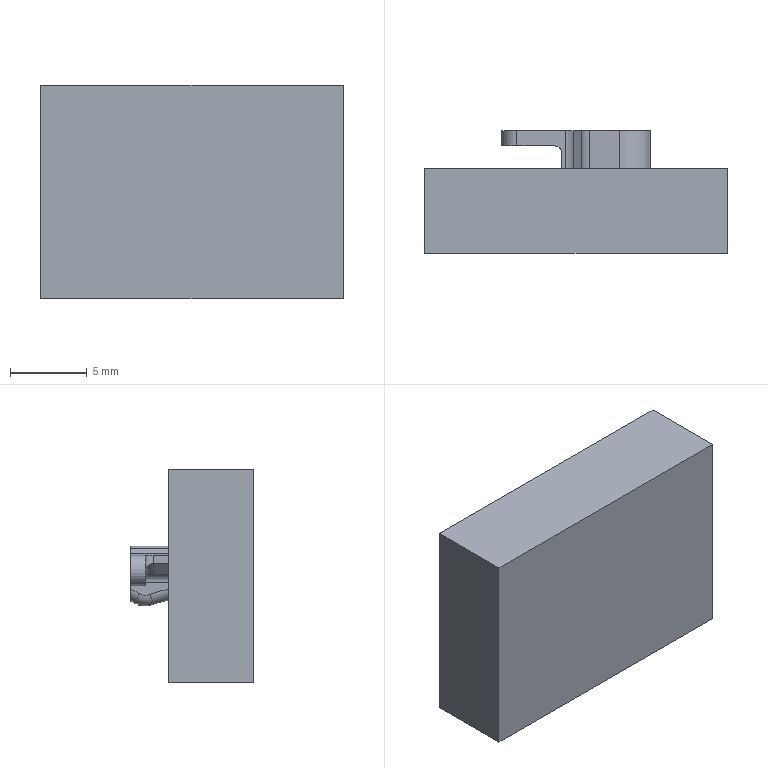NC program | NX | posted with a generic post | part box 19.7 x 8 x 13.91 mm
Lines 1 to 1448 of 12456:
N10 G17 G21 G94 G90
(CAVITY_MILL , TOOL : D3)
N12 T03 M6
N14 G54
N16 G17 G0 G90 X11.774 Y-0.48 B0. C0. S5000 M3
N18 G43 Z30. H3
N20 Z0.07
N22 G94 G1 Z-0.93 F1000.
N24 X10.679 Y-0.359
N26 G2 X9.684 Y-0.457 R1.
N28 G1 X9.673 Y-0.452 F1500.
N30 X9.664 Y-0.45
N32 X9.223
N34 X9.175
N36 X9.031
N38 X8.788
N40 X8.544
N42 X7.309
N44 Y0.46
N46 X8.057 Y0.461
N48 X8.301 Y0.46
N50 X8.544 Y0.461
N52 X8.788
N54 X9.031 Y0.46
N56 X9.205
N58 X9.392 Y0.461
N60 X9.518
N62 X9.558
N64 X9.687 Y0.452
N66 X9.708 Y0.449
N68 X9.709 Y0.47
N70 Y0.48
N72 X9.712 Y0.501
N74 X9.691 Y0.502
N76 X9.559 Y0.511
N78 X9.518
N80 X9.392
N82 X9.205
N84 X9.031
N86 X8.788 Y0.513
N88 X8.544
N90 X8.301 Y0.512
N92 X8.057 Y0.511
N94 X7.328 Y0.51
N96 X7.299 Y0.511
N98 X7.083 Y0.5
N100 X6.596
N102 X6.353
N104 X5.977
N106 X5.866
N108 X5.778
N110 X5.757 Y0.501
N112 X5.758 Y0.48
N114 Y-0.48
N116 X5.757 Y-0.501
N118 X5.778 Y-0.5
N120 X5.866
N122 X5.977
N124 X6.353
N126 X6.596
N128 X8.301
N130 X8.544
N132 X8.788
N134 X9.031
N136 X9.686
N138 X9.71 Y-0.499
N140 X9.716 Y-0.473
N142 X9.695 Y-0.462
N144 X9.684 Y-0.457
N146 G2 X9.101 Y0.356 R1.
N148 G1 Z0.07
N150 G0 Z30.
N152 X11.774 Y-0.48
N154 Z0.05
N156 G1 Z-0.95 F1000.
N158 X10.679 Y-0.359
N160 G2 X9.684 Y-0.457 R1.
N162 G1 X9.673 Y-0.452 F1500.
N164 X9.664 Y-0.45
N166 X9.223
N168 X9.175
N170 X9.031
N172 X8.788
N174 X8.544
N176 X7.309
N178 Y0.46
N180 X8.057 Y0.461
N182 X8.301 Y0.46
N184 X8.544 Y0.461
N186 X8.788
N188 X9.031 Y0.46
N190 X9.205
N192 X9.392 Y0.461
N194 X9.518
N196 X9.558
N198 X9.687 Y0.452
N200 X9.708 Y0.449
N202 X9.709 Y0.47
N204 Y0.48
N206 X9.712 Y0.501
N208 X9.691 Y0.502
N210 X9.559 Y0.511
N212 X9.518
N214 X9.392
N216 X9.205
N218 X9.031
N220 X8.788 Y0.513
N222 X8.544
N224 X8.301 Y0.512
N226 X8.057 Y0.511
N228 X7.328 Y0.51
N230 X7.299 Y0.511
N232 X7.083 Y0.5
N234 X6.596
N236 X6.353
N238 X5.977
N240 X5.866
N242 X5.778
N244 X5.757 Y0.501
N246 X5.758 Y0.48
N248 Y-0.48
N250 X5.757 Y-0.501
N252 X5.778 Y-0.5
N254 X5.866
N256 X5.977
N258 X6.353
N260 X6.596
N262 X8.301
N264 X8.544
N266 X8.788
N268 X9.031
N270 X9.686
N272 X9.71 Y-0.499
N274 X9.716 Y-0.473
N276 X9.695 Y-0.462
N278 X9.684 Y-0.457
N280 G2 X9.101 Y0.356 R1.
N282 G1 Z0.05
N284 G0 Z30.
N286 X11.774 Y-0.48
N288 Z0.03
N290 G1 Z-0.97 F1000.
N292 X10.679 Y-0.359
N294 G2 X9.684 Y-0.457 R1.
N296 G1 X9.673 Y-0.452 F1500.
N298 X9.664 Y-0.45
N300 X9.223
N302 X9.175
N304 X9.031
N306 X8.788
N308 X8.544
N310 X7.309
N312 Y0.46
N314 X8.057 Y0.461
N316 X8.301 Y0.46
N318 X8.544 Y0.461
N320 X8.788
N322 X9.031 Y0.46
N324 X9.205
N326 X9.392 Y0.461
N328 X9.518
N330 X9.558
N332 X9.687 Y0.452
N334 X9.708 Y0.449
N336 X9.709 Y0.47
N338 Y0.48
N340 X9.712 Y0.501
N342 X9.691 Y0.502
N344 X9.559 Y0.511
N346 X9.518
N348 X9.392
N350 X9.205
N352 X9.031
N354 X8.788 Y0.513
N356 X8.544
N358 X8.301 Y0.512
N360 X8.057 Y0.511
N362 X7.328 Y0.51
N364 X7.299 Y0.511
N366 X7.083 Y0.5
N368 X6.596
N370 X6.353
N372 X5.977
N374 X5.866
N376 X5.778
N378 X5.757 Y0.501
N380 X5.758 Y0.48
N382 Y-0.48
N384 X5.757 Y-0.501
N386 X5.778 Y-0.5
N388 X5.866
N390 X5.977
N392 X6.353
N394 X6.596
N396 X8.301
N398 X8.544
N400 X8.788
N402 X9.031
N404 X9.686
N406 X9.71 Y-0.499
N408 X9.716 Y-0.473
N410 X9.695 Y-0.462
N412 X9.684 Y-0.457
N414 G2 X9.101 Y0.356 R1.
N416 G1 Z0.03
N418 G0 Z30.
N420 X11.774 Y-0.48
N422 Z0.01
N424 G1 Z-0.99 F1000.
N426 X10.679 Y-0.359
N428 G2 X9.684 Y-0.457 R1.
N430 G1 X9.673 Y-0.452 F1500.
N432 X9.664 Y-0.45
N434 X9.223
N436 X9.175
N438 X9.031
N440 X8.788
N442 X8.544
N444 X7.309
N446 Y0.46
N448 X8.057 Y0.461
N450 X8.301 Y0.46
N452 X8.544 Y0.461
N454 X8.788
N456 X9.031 Y0.46
N458 X9.205
N460 X9.392 Y0.461
N462 X9.518
N464 X9.558
N466 X9.687 Y0.452
N468 X9.708 Y0.449
N470 X9.709 Y0.47
N472 Y0.48
N474 X9.712 Y0.501
N476 X9.691 Y0.502
N478 X9.559 Y0.511
N480 X9.518
N482 X9.392
N484 X9.205
N486 X9.031
N488 X8.788 Y0.513
N490 X8.544
N492 X8.301 Y0.512
N494 X8.057 Y0.511
N496 X7.328 Y0.51
N498 X7.299 Y0.511
N500 X7.083 Y0.5
N502 X6.596
N504 X6.353
N506 X5.977
N508 X5.866
N510 X5.778
N512 X5.757 Y0.501
N514 X5.758 Y0.48
N516 Y-0.48
N518 X5.757 Y-0.501
N520 X5.778 Y-0.5
N522 X5.866
N524 X5.977
N526 X6.353
N528 X6.596
N530 X8.301
N532 X8.544
N534 X8.788
N536 X9.031
N538 X9.686
N540 X9.71 Y-0.499
N542 X9.716 Y-0.473
N544 X9.695 Y-0.462
N546 X9.684 Y-0.457
N548 G2 X9.101 Y0.356 R1.
N550 G1 Z0.01
N552 G0 Z30.
N554 X11.774 Y-0.48
N556 Z-0.01
N558 G1 Z-1.01 F1000.
N560 X10.679 Y-0.359
N562 G2 X9.684 Y-0.457 R1.
N564 G1 X9.673 Y-0.452 F1500.
N566 X9.664 Y-0.45
N568 X9.223
N570 X9.175
N572 X9.031
N574 X8.788
N576 X8.544
N578 X7.309
N580 Y0.46
N582 X8.057 Y0.461
N584 X8.301 Y0.46
N586 X8.544 Y0.461
N588 X8.788
N590 X9.031 Y0.46
N592 X9.205
N594 X9.392 Y0.461
N596 X9.518
N598 X9.558
N600 X9.687 Y0.452
N602 X9.708 Y0.449
N604 X9.709 Y0.47
N606 Y0.48
N608 X9.712 Y0.501
N610 X9.691 Y0.502
N612 X9.559 Y0.511
N614 X9.518
N616 X9.392
N618 X9.205
N620 X9.031
N622 X8.788 Y0.513
N624 X8.544
N626 X8.301 Y0.512
N628 X8.057 Y0.511
N630 X7.328 Y0.51
N632 X7.299 Y0.511
N634 X7.083 Y0.5
N636 X6.596
N638 X6.353
N640 X5.977
N642 X5.866
N644 X5.778
N646 X5.757 Y0.501
N648 X5.758 Y0.48
N650 Y-0.48
N652 X5.757 Y-0.501
N654 X5.778 Y-0.5
N656 X5.866
N658 X5.977
N660 X6.353
N662 X6.596
N664 X8.301
N666 X8.544
N668 X8.788
N670 X9.031
N672 X9.686
N674 X9.71 Y-0.499
N676 X9.716 Y-0.473
N678 X9.695 Y-0.462
N680 X9.684 Y-0.457
N682 G2 X9.101 Y0.356 R1.
N684 G1 Z-0.01
N686 G0 Z30.
N688 X11.774 Y-0.48
N690 Z-0.03
N692 G1 Z-1.03 F1000.
N694 X10.679 Y-0.359
N696 G2 X9.684 Y-0.457 R1.
N698 G1 X9.673 Y-0.452 F1500.
N700 X9.664 Y-0.45
N702 X9.223
N704 X9.175
N706 X9.031
N708 X8.788
N710 X8.544
N712 X7.309
N714 Y0.46
N716 X8.057 Y0.461
N718 X8.301 Y0.46
N720 X8.544 Y0.461
N722 X8.788
N724 X9.031 Y0.46
N726 X9.205
N728 X9.392 Y0.461
N730 X9.518
N732 X9.558
N734 X9.687 Y0.452
N736 X9.708 Y0.449
N738 X9.709 Y0.47
N740 Y0.48
N742 X9.712 Y0.501
N744 X9.691 Y0.502
N746 X9.559 Y0.511
N748 X9.518
N750 X9.392
N752 X9.205
N754 X9.031
N756 X8.788 Y0.513
N758 X8.544
N760 X8.301 Y0.512
N762 X8.057 Y0.511
N764 X7.328 Y0.51
N766 X7.299 Y0.511
N768 X7.083 Y0.5
N770 X6.596
N772 X6.353
N774 X5.977
N776 X5.866
N778 X5.778
N780 X5.757 Y0.501
N782 X5.758 Y0.48
N784 Y-0.48
N786 X5.757 Y-0.501
N788 X5.778 Y-0.5
N790 X5.866
N792 X5.977
N794 X6.353
N796 X6.596
N798 X8.301
N800 X8.544
N802 X8.788
N804 X9.031
N806 X9.686
N808 X9.71 Y-0.499
N810 X9.716 Y-0.473
N812 X9.695 Y-0.462
N814 X9.684 Y-0.457
N816 G2 X9.101 Y0.356 R1.
N818 G1 Z-0.03
N820 G0 Z30.
N822 X11.774 Y-0.48
N824 Z-0.05
N826 G1 Z-1.05 F1000.
N828 X10.679 Y-0.359
N830 G2 X9.684 Y-0.457 R1.
N832 G1 X9.673 Y-0.452 F1500.
N834 X9.664 Y-0.45
N836 X9.223
N838 X9.175
N840 X9.031
N842 X8.788
N844 X8.544
N846 X7.309
N848 Y0.46
N850 X8.057 Y0.461
N852 X8.301 Y0.46
N854 X8.544 Y0.461
N856 X8.788
N858 X9.031 Y0.46
N860 X9.205
N862 X9.392 Y0.461
N864 X9.518
N866 X9.558
N868 X9.687 Y0.452
N870 X9.708 Y0.449
N872 X9.709 Y0.47
N874 Y0.48
N876 X9.712 Y0.501
N878 X9.691 Y0.502
N880 X9.559 Y0.511
N882 X9.518
N884 X9.392
N886 X9.205
N888 X9.031
N890 X8.788 Y0.513
N892 X8.544
N894 X8.301 Y0.512
N896 X8.057 Y0.511
N898 X7.328 Y0.51
N900 X7.299 Y0.511
N902 X7.083 Y0.5
N904 X6.596
N906 X6.353
N908 X5.977
N910 X5.866
N912 X5.778
N914 X5.757 Y0.501
N916 X5.758 Y0.48
N918 Y-0.48
N920 X5.757 Y-0.501
N922 X5.778 Y-0.5
N924 X5.866
N926 X5.977
N928 X6.353
N930 X6.596
N932 X8.301
N934 X8.544
N936 X8.788
N938 X9.031
N940 X9.686
N942 X9.71 Y-0.499
N944 X9.716 Y-0.473
N946 X9.695 Y-0.462
N948 X9.684 Y-0.457
N950 G2 X9.101 Y0.356 R1.
N952 G1 Z-0.05
N954 G0 Z30.
N956 X11.774 Y-0.48
N958 Z-0.07
N960 G1 Z-1.07 F1000.
N962 X10.679 Y-0.359
N964 G2 X9.684 Y-0.457 R1.
N966 G1 X9.673 Y-0.452 F1500.
N968 X9.664 Y-0.45
N970 X9.223
N972 X9.175
N974 X9.031
N976 X8.788
N978 X8.544
N980 X7.309
N982 Y0.46
N984 X8.057 Y0.461
N986 X8.301 Y0.46
N988 X8.544 Y0.461
N990 X8.788
N992 X9.031 Y0.46
N994 X9.205
N996 X9.392 Y0.461
N998 X9.518
N1000 X9.558
N1002 X9.687 Y0.452
N1004 X9.708 Y0.449
N1006 X9.709 Y0.47
N1008 Y0.48
N1010 X9.712 Y0.501
N1012 X9.691 Y0.502
N1014 X9.559 Y0.511
N1016 X9.518
N1018 X9.392
N1020 X9.205
N1022 X9.031
N1024 X8.788 Y0.513
N1026 X8.544
N1028 X8.301 Y0.512
N1030 X8.057 Y0.511
N1032 X7.328 Y0.51
N1034 X7.299 Y0.511
N1036 X7.083 Y0.5
N1038 X6.596
N1040 X6.353
N1042 X5.977
N1044 X5.866
N1046 X5.778
N1048 X5.757 Y0.501
N1050 X5.758 Y0.48
N1052 Y-0.48
N1054 X5.757 Y-0.501
N1056 X5.778 Y-0.5
N1058 X5.866
N1060 X5.977
N1062 X6.353
N1064 X6.596
N1066 X8.301
N1068 X8.544
N1070 X8.788
N1072 X9.031
N1074 X9.686
N1076 X9.71 Y-0.499
N1078 X9.716 Y-0.473
N1080 X9.695 Y-0.462
N1082 X9.684 Y-0.457
N1084 G2 X9.101 Y0.356 R1.
N1086 G1 Z-0.07
N1088 G0 Z30.
N1090 X11.774 Y-0.48
N1092 Z-0.09
N1094 G1 Z-1.09 F1000.
N1096 X10.679 Y-0.359
N1098 G2 X9.684 Y-0.457 R1.
N1100 G1 X9.673 Y-0.452 F1500.
N1102 X9.664 Y-0.45
N1104 X9.223
N1106 X9.175
N1108 X9.031
N1110 X8.788
N1112 X8.544
N1114 X7.309
N1116 Y0.46
N1118 X8.057 Y0.461
N1120 X8.301 Y0.46
N1122 X8.544 Y0.461
N1124 X8.788
N1126 X9.031 Y0.46
N1128 X9.205
N1130 X9.392 Y0.461
N1132 X9.518
N1134 X9.558
N1136 X9.687 Y0.452
N1138 X9.708 Y0.449
N1140 X9.709 Y0.47
N1142 Y0.48
N1144 X9.712 Y0.501
N1146 X9.691 Y0.502
N1148 X9.559 Y0.511
N1150 X9.518
N1152 X9.392
N1154 X9.205
N1156 X9.031
N1158 X8.788 Y0.513
N1160 X8.544
N1162 X8.301 Y0.512
N1164 X8.057 Y0.511
N1166 X7.328 Y0.51
N1168 X7.299 Y0.511
N1170 X7.083 Y0.5
N1172 X6.596
N1174 X6.353
N1176 X5.977
N1178 X5.866
N1180 X5.778
N1182 X5.757 Y0.501
N1184 X5.758 Y0.48
N1186 Y-0.48
N1188 X5.757 Y-0.501
N1190 X5.778 Y-0.5
N1192 X5.866
N1194 X5.977
N1196 X6.353
N1198 X6.596
N1200 X8.301
N1202 X8.544
N1204 X8.788
N1206 X9.031
N1208 X9.686
N1210 X9.71 Y-0.499
N1212 X9.716 Y-0.473
N1214 X9.695 Y-0.462
N1216 X9.684 Y-0.457
N1218 G2 X9.101 Y0.356 R1.
N1220 G1 Z-0.09
N1222 G0 Z30.
N1224 X11.774 Y-0.48
N1226 Z-0.11
N1228 G1 Z-1.11 F1000.
N1230 X10.679 Y-0.359
N1232 G2 X9.684 Y-0.457 R1.
N1234 G1 X9.673 Y-0.452 F1500.
N1236 X9.664 Y-0.45
N1238 X9.223
N1240 X9.175
N1242 X9.031
N1244 X8.788
N1246 X8.544
N1248 X7.309
N1250 Y0.46
N1252 X8.057 Y0.461
N1254 X8.301 Y0.46
N1256 X8.544 Y0.461
N1258 X8.788
N1260 X9.031 Y0.46
N1262 X9.205
N1264 X9.392 Y0.461
N1266 X9.518
N1268 X9.558
N1270 X9.687 Y0.452
N1272 X9.708 Y0.449
N1274 X9.709 Y0.47
N1276 Y0.48
N1278 X9.712 Y0.501
N1280 X9.691 Y0.502
N1282 X9.559 Y0.511
N1284 X9.518
N1286 X9.392
N1288 X9.205
N1290 X9.031
N1292 X8.788 Y0.513
N1294 X8.544
N1296 X8.301 Y0.512
N1298 X8.057 Y0.511
N1300 X7.328 Y0.51
N1302 X7.299 Y0.511
N1304 X7.083 Y0.5
N1306 X6.596
N1308 X6.353
N1310 X5.977
N1312 X5.866
N1314 X5.778
N1316 X5.757 Y0.501
N1318 X5.758 Y0.48
N1320 Y-0.48
N1322 X5.757 Y-0.501
N1324 X5.778 Y-0.5
N1326 X5.866
N1328 X5.977
N1330 X6.353
N1332 X6.596
N1334 X8.301
N1336 X8.544
N1338 X8.788
N1340 X9.031
N1342 X9.686
N1344 X9.71 Y-0.499
N1346 X9.716 Y-0.473
N1348 X9.695 Y-0.462
N1350 X9.684 Y-0.457
N1352 G2 X9.101 Y0.356 R1.
N1354 G1 Z-0.11
N1356 G0 Z30.
N1358 X11.774 Y-0.48
N1360 Z-0.13
N1362 G1 Z-1.13 F1000.
N1364 X10.679 Y-0.359
N1366 G2 X9.684 Y-0.457 R1.
N1368 G1 X9.673 Y-0.452 F1500.
N1370 X9.664 Y-0.45
N1372 X9.223
N1374 X9.175
N1376 X9.031
N1378 X8.788
N1380 X8.544
N1382 X7.309
N1384 Y0.46
N1386 X8.057 Y0.461
N1388 X8.301 Y0.46
N1390 X8.544 Y0.461
N1392 X8.788
N1394 X9.031 Y0.46
N1396 X9.205
N1398 X9.392 Y0.461
N1400 X9.518
N1402 X9.558
N1404 X9.687 Y0.452
N1406 X9.708 Y0.449
N1408 X9.709 Y0.47
N1410 Y0.48
N1412 X9.712 Y0.501
N1414 X9.691 Y0.502
N1416 X9.559 Y0.511
N1418 X9.518
N1420 X9.392
N1422 X9.205
N1424 X9.031
N1426 X8.788 Y0.513
N1428 X8.544
N1430 X8.301 Y0.512
N1432 X8.057 Y0.511
N1434 X7.328 Y0.51
N1436 X7.299 Y0.511
N1438 X7.083 Y0.5
N1440 X6.596
N1442 X6.353
N1444 X5.977
N1446 X5.866
N1448 X5.778
N1450 X5.757 Y0.501
N1452 X5.758 Y0.48
N1454 Y-0.48
N1456 X5.757 Y-0.501
N1458 X5.778 Y-0.5
N1460 X5.866
N1462 X5.977
N1464 X6.353
N1466 X6.596
N1468 X8.301
N1470 X8.544
N1472 X8.788
N1474 X9.031
N1476 X9.686
N1478 X9.71 Y-0.499
N1480 X9.716 Y-0.473
N1482 X9.695 Y-0.462
N1484 X9.684 Y-0.457
N1486 G2 X9.101 Y0.356 R1.
N1488 G1 Z-0.13
N1490 G0 Z30.
N1492 X11.774 Y-0.48
N1494 Z-0.15
N1496 G1 Z-1.15 F1000.
N1498 X10.679 Y-0.359
N1500 G2 X9.684 Y-0.457 R1.
N1502 G1 X9.673 Y-0.452 F1500.
N1504 X9.664 Y-0.45
N1506 X9.223
N1508 X9.175
N1510 X9.031
N1512 X8.788
N1514 X8.544
N1516 X7.309
N1518 Y0.46
N1520 X8.057 Y0.461
N1522 X8.301 Y0.46
N1524 X8.544 Y0.461
N1526 X8.788
N1528 X9.031 Y0.46
N1530 X9.205
N1532 X9.392 Y0.461
N1534 X9.518
N1536 X9.558
N1538 X9.687 Y0.452
N1540 X9.708 Y0.449
N1542 X9.709 Y0.47
N1544 Y0.48
N1546 X9.712 Y0.501
N1548 X9.691 Y0.502
N1550 X9.559 Y0.511
N1552 X9.518
N1554 X9.392
N1556 X9.205
N1558 X9.031
N1560 X8.788 Y0.513
N1562 X8.544
N1564 X8.301 Y0.512
N1566 X8.057 Y0.511
N1568 X7.328 Y0.51
N1570 X7.299 Y0.511
N1572 X7.083 Y0.5
N1574 X6.596
N1576 X6.353
N1578 X5.977
N1580 X5.866
N1582 X5.778
N1584 X5.757 Y0.501
N1586 X5.758 Y0.48
N1588 Y-0.48
N1590 X5.757 Y-0.501
N1592 X5.778 Y-0.5
N1594 X5.866
N1596 X5.977
N1598 X6.353
N1600 X6.596
N1602 X8.301
N1604 X8.544
N1606 X8.788
N1608 X9.031
N1610 X9.686
N1612 X9.71 Y-0.499
N1614 X9.716 Y-0.473
N1616 X9.695 Y-0.462
N1618 X9.684 Y-0.457
N1620 G2 X9.101 Y0.356 R1.
N1622 G1 Z-0.15
N1624 G0 Z30.
N1626 X11.774 Y-0.48
N1628 Z-0.17
N1630 G1 Z-1.17 F1000.
N1632 X10.679 Y-0.359
N1634 G2 X9.684 Y-0.457 R1.
N1636 G1 X9.673 Y-0.452 F1500.
N1638 X9.664 Y-0.45
N1640 X9.223
N1642 X9.175
N1644 X9.031
N1646 X8.788
N1648 X8.544
N1650 X7.309
N1652 Y0.46
N1654 X8.057 Y0.461
N1656 X8.301 Y0.46
N1658 X8.544 Y0.461
N1660 X8.788
N1662 X9.031 Y0.46
N1664 X9.205
N1666 X9.392 Y0.461
N1668 X9.518
N1670 X9.558
N1672 X9.687 Y0.452
N1674 X9.708 Y0.449
N1676 X9.709 Y0.47
N1678 Y0.48
N1680 X9.712 Y0.501
N1682 X9.691 Y0.502
N1684 X9.559 Y0.511
N1686 X9.518
N1688 X9.392
N1690 X9.205
N1692 X9.031
N1694 X8.788 Y0.513
N1696 X8.544
N1698 X8.301 Y0.512
N1700 X8.057 Y0.511
N1702 X7.328 Y0.51
N1704 X7.299 Y0.511
N1706 X7.083 Y0.5
N1708 X6.596
N1710 X6.353
N1712 X5.977
N1714 X5.866
N1716 X5.778
N1718 X5.757 Y0.501
N1720 X5.758 Y0.48
N1722 Y-0.48
N1724 X5.757 Y-0.501
N1726 X5.778 Y-0.5
N1728 X5.866
N1730 X5.977
N1732 X6.353
N1734 X6.596
N1736 X8.301
N1738 X8.544
N1740 X8.788
N1742 X9.031
N1744 X9.686
N1746 X9.71 Y-0.499
N1748 X9.716 Y-0.473
N1750 X9.695 Y-0.462
N1752 X9.684 Y-0.457
N1754 G2 X9.101 Y0.356 R1.
N1756 G1 Z-0.17
N1758 G0 Z30.
N1760 X11.774 Y-0.48
N1762 Z-0.19
N1764 G1 Z-1.19 F1000.
N1766 X10.679 Y-0.359
N1768 G2 X9.684 Y-0.457 R1.
N1770 G1 X9.673 Y-0.452 F1500.
N1772 X9.664 Y-0.45
N1774 X9.223
N1776 X9.175
N1778 X9.031
N1780 X8.788
N1782 X8.544
N1784 X7.309
N1786 Y0.46
N1788 X8.057 Y0.461
N1790 X8.301 Y0.46
N1792 X8.544 Y0.461
N1794 X8.788
N1796 X9.031 Y0.46
N1798 X9.205
N1800 X9.392 Y0.461
N1802 X9.518
N1804 X9.558
N1806 X9.687 Y0.452
N1808 X9.708 Y0.449
N1810 X9.709 Y0.47
N1812 Y0.48
N1814 X9.712 Y0.501
N1816 X9.691 Y0.502
N1818 X9.559 Y0.511
N1820 X9.518
N1822 X9.392
N1824 X9.205
N1826 X9.031
N1828 X8.788 Y0.513
N1830 X8.544
N1832 X8.301 Y0.512
N1834 X8.057 Y0.511
N1836 X7.328 Y0.51
N1838 X7.299 Y0.511
N1840 X7.083 Y0.5
N1842 X6.596
N1844 X6.353
N1846 X5.977
N1848 X5.866
N1850 X5.778
N1852 X5.757 Y0.501
N1854 X5.758 Y0.48
N1856 Y-0.48
N1858 X5.757 Y-0.501
N1860 X5.778 Y-0.5
N1862 X5.866
N1864 X5.977
N1866 X6.353
N1868 X6.596
N1870 X8.301
N1872 X8.544
N1874 X8.788
N1876 X9.031
N1878 X9.686
N1880 X9.71 Y-0.499
N1882 X9.716 Y-0.473
N1884 X9.695 Y-0.462
N1886 X9.684 Y-0.457
N1888 G2 X9.101 Y0.356 R1.
N1890 G1 Z-0.19
N1892 G0 Z30.
N1894 X11.775 Y-0.48
N1896 Z-0.21
N1898 G1 Z-1.21 F1000.
N1900 X10.679 Y-0.359
N1902 G2 X9.684 Y-0.457 R1.
N1904 G1 X9.673 Y-0.452 F1500.
N1906 X9.664 Y-0.45
N1908 X9.223
N1910 X9.175
N1912 X9.031
N1914 X8.788
N1916 X8.544
N1918 X7.309
N1920 Y0.46
N1922 X8.057 Y0.461
N1924 X8.301 Y0.46
N1926 X8.544 Y0.461
N1928 X8.788
N1930 X9.031 Y0.46
N1932 X9.205
N1934 X9.392 Y0.461
N1936 X9.518
N1938 X9.558
N1940 X9.687 Y0.452
N1942 X9.708 Y0.449
N1944 X9.709 Y0.47
N1946 Y0.48
N1948 X9.712 Y0.501
N1950 X9.691 Y0.502
N1952 X9.559 Y0.511
N1954 X9.518
N1956 X9.392
N1958 X9.205
N1960 X9.031
N1962 X8.788 Y0.513
N1964 X8.544
N1966 X8.301 Y0.512
N1968 X8.057 Y0.511
N1970 X7.328 Y0.51
N1972 X7.299 Y0.511
N1974 X7.083 Y0.5
N1976 X6.596
N1978 X6.353
N1980 X5.977
N1982 X5.866
N1984 X5.778
N1986 X5.757 Y0.501
N1988 X5.758 Y0.48
N1990 Y-0.48
N1992 X5.757 Y-0.501
N1994 X5.778 Y-0.5
N1996 X5.866
N1998 X5.977
N2000 X6.353
N2002 X6.596
N2004 X8.301
N2006 X8.544
N2008 X8.788
N2010 X9.031
N2012 X9.686
N2014 X9.71 Y-0.499
N2016 X9.716 Y-0.473
N2018 X9.695 Y-0.462
N2020 X9.684 Y-0.457
N2022 G2 X9.101 Y0.356 R1.
N2024 G1 Z-0.21
N2026 G0 Z30.
N2028 X11.775 Y-0.48
N2030 Z-0.23
N2032 G1 Z-1.23 F1000.
N2034 X10.679 Y-0.359
N2036 G2 X9.684 Y-0.457 R1.
N2038 G1 X9.673 Y-0.452 F1500.
N2040 X9.664 Y-0.45
N2042 X9.223
N2044 X9.175
N2046 X9.031
N2048 X8.788
N2050 X8.544
N2052 X7.309
N2054 Y0.46
N2056 X8.057 Y0.461
N2058 X8.301 Y0.46
N2060 X8.544 Y0.461
N2062 X8.788
N2064 X9.031 Y0.46
N2066 X9.205
N2068 X9.392 Y0.461
N2070 X9.518
N2072 X9.558
N2074 X9.687 Y0.452
N2076 X9.708 Y0.449
N2078 X9.709 Y0.47
N2080 Y0.48
N2082 X9.712 Y0.501
N2084 X9.691 Y0.502
N2086 X9.559 Y0.511
N2088 X9.518
N2090 X9.392
N2092 X9.205
N2094 X9.031
N2096 X8.788 Y0.513
N2098 X8.544
N2100 X8.301 Y0.512
N2102 X8.057 Y0.511
N2104 X7.328 Y0.51
N2106 X7.299 Y0.511
N2108 X7.083 Y0.5
N2110 X6.596
N2112 X6.353
N2114 X5.977
N2116 X5.866
N2118 X5.778
N2120 X5.757 Y0.501
N2122 X5.758 Y0.48
N2124 Y-0.48
N2126 X5.757 Y-0.501
N2128 X5.778 Y-0.5
N2130 X5.866
N2132 X5.977
N2134 X6.353
N2136 X6.596
N2138 X8.301
N2140 X8.544
N2142 X8.788
N2144 X9.031
N2146 X9.686
N2148 X9.71 Y-0.499
N2150 X9.716 Y-0.473
N2152 X9.695 Y-0.462
N2154 X9.684 Y-0.457
N2156 G2 X9.101 Y0.356 R1.
N2158 G1 Z-0.23
N2160 G0 Z30.
N2162 X11.775 Y-0.48
N2164 Z-0.25
N2166 G1 Z-1.25 F1000.
N2168 X10.679 Y-0.359
N2170 G2 X9.684 Y-0.457 R1.
N2172 G1 X9.673 Y-0.452 F1500.
N2174 X9.664 Y-0.45
N2176 X9.223
N2178 X9.175
N2180 X9.031
N2182 X8.788
N2184 X8.544
N2186 X7.309
N2188 Y0.46
N2190 X8.057 Y0.461
N2192 X8.301 Y0.46
N2194 X8.544 Y0.461
N2196 X8.788
N2198 X9.031 Y0.46
N2200 X9.205
N2202 X9.392 Y0.461
N2204 X9.518
N2206 X9.558
N2208 X9.687 Y0.452
N2210 X9.708 Y0.449
N2212 X9.709 Y0.47
N2214 Y0.48
N2216 X9.712 Y0.501
N2218 X9.691 Y0.502
N2220 X9.559 Y0.511
N2222 X9.518
N2224 X9.392
N2226 X9.205
N2228 X9.031
N2230 X8.788 Y0.513
N2232 X8.544
N2234 X8.301 Y0.512
N2236 X8.057 Y0.511
N2238 X7.328 Y0.51
N2240 X7.299 Y0.511
N2242 X7.083 Y0.5
N2244 X6.596
N2246 X6.353
N2248 X5.977
N2250 X5.866
N2252 X5.778
N2254 X5.757 Y0.501
N2256 X5.758 Y0.48
N2258 Y-0.48
N2260 X5.757 Y-0.501
N2262 X5.778 Y-0.5
N2264 X5.866
N2266 X5.977
N2268 X6.353
N2270 X6.596
N2272 X8.301
N2274 X8.544
N2276 X8.788
N2278 X9.031
N2280 X9.686
N2282 X9.71 Y-0.499
N2284 X9.716 Y-0.473
N2286 X9.695 Y-0.462
N2288 X9.684 Y-0.457
N2290 G2 X9.101 Y0.356 R1.
N2292 G1 Z-0.25
N2294 G0 Z30.
N2296 X11.775 Y-0.48
N2298 Z-0.27
N2300 G1 Z-1.27 F1000.
N2302 X10.679 Y-0.359
N2304 G2 X9.684 Y-0.457 R1.
N2306 G1 X9.673 Y-0.452 F1500.
N2308 X9.664 Y-0.45
N2310 X9.223
N2312 X9.175
N2314 X9.031
N2316 X8.788
N2318 X8.544
N2320 X7.309
N2322 Y0.46
N2324 X8.057 Y0.461
N2326 X8.301 Y0.46
N2328 X8.544 Y0.461
N2330 X8.788
N2332 X9.031 Y0.46
N2334 X9.205
N2336 X9.392 Y0.461
N2338 X9.518
N2340 X9.558
N2342 X9.687 Y0.452
N2344 X9.708 Y0.449
N2346 X9.709 Y0.47
N2348 Y0.48
N2350 X9.712 Y0.501
N2352 X9.691 Y0.502
N2354 X9.559 Y0.511
N2356 X9.518
N2358 X9.392
N2360 X9.205
N2362 X9.031
N2364 X8.788 Y0.513
N2366 X8.544
N2368 X8.301 Y0.512
N2370 X8.057 Y0.511
N2372 X7.328 Y0.51
N2374 X7.299 Y0.511
N2376 X7.083 Y0.5
N2378 X6.596
N2380 X6.353
N2382 X5.977
N2384 X5.866
N2386 X5.778
N2388 X5.757 Y0.501
N2390 X5.758 Y0.48
N2392 Y-0.48
N2394 X5.757 Y-0.501
N2396 X5.778 Y-0.5
N2398 X5.866
N2400 X5.977
N2402 X6.353
N2404 X6.596
N2406 X8.301
N2408 X8.544
N2410 X8.788
N2412 X9.031
N2414 X9.686
N2416 X9.71 Y-0.499
N2418 X9.716 Y-0.473
N2420 X9.695 Y-0.462
N2422 X9.684 Y-0.457
N2424 G2 X9.101 Y0.356 R1.
N2426 G1 Z-0.27
N2428 G0 Z30.
N2430 X11.775 Y-0.48
N2432 Z-0.29
N2434 G1 Z-1.29 F1000.
N2436 X10.679 Y-0.359
N2438 G2 X9.684 Y-0.457 R1.
N2440 G1 X9.673 Y-0.452 F1500.
N2442 X9.664 Y-0.45
N2444 X9.223
N2446 X9.175
N2448 X9.031
N2450 X8.788
N2452 X8.544
N2454 X7.309
N2456 Y0.46
N2458 X8.057 Y0.461
N2460 X8.301 Y0.46
N2462 X8.544 Y0.461
N2464 X8.788
N2466 X9.031 Y0.46
N2468 X9.205
N2470 X9.392 Y0.461
N2472 X9.518
N2474 X9.558
N2476 X9.687 Y0.452
N2478 X9.708 Y0.449
N2480 X9.709 Y0.47
N2482 Y0.48
N2484 X9.712 Y0.501
N2486 X9.691 Y0.502
N2488 X9.559 Y0.511
N2490 X9.518
N2492 X9.392
N2494 X9.205
N2496 X9.031
N2498 X8.788 Y0.513
N2500 X8.544
N2502 X8.301 Y0.512
N2504 X8.057 Y0.511
N2506 X7.328 Y0.51
N2508 X7.299 Y0.511
N2510 X7.083 Y0.5
N2512 X6.596
N2514 X6.353
N2516 X5.977
N2518 X5.866
N2520 X5.778
N2522 X5.757 Y0.501
N2524 X5.758 Y0.48
N2526 Y-0.48
N2528 X5.757 Y-0.501
N2530 X5.778 Y-0.5
N2532 X5.866
N2534 X5.977
N2536 X6.353
N2538 X6.596
N2540 X8.301
N2542 X8.533
N2544 G2 X8.92 Y-0.5 R1.297
N2546 G1 X9.031
N2548 X9.686
N2550 X9.71 Y-0.499
N2552 X9.716 Y-0.473
N2554 X9.695 Y-0.462
N2556 X9.684 Y-0.457
N2558 G2 X9.101 Y0.356 R1.
N2560 G1 Z-0.29
N2562 G0 Z30.
N2564 X11.775 Y-0.48
N2566 Z-0.31
N2568 G1 Z-1.31 F1000.
N2570 X10.679 Y-0.359
N2572 G2 X9.684 Y-0.457 R1.
N2574 G1 X9.673 Y-0.452 F1500.
N2576 X9.664 Y-0.45
N2578 X9.223
N2580 X9.175
N2582 X9.031
N2584 X8.788
N2586 X8.544
N2588 X7.309
N2590 Y0.46
N2592 X8.057 Y0.461
N2594 X8.301 Y0.46
N2596 X8.544 Y0.461
N2598 X8.788
N2600 X9.031 Y0.46
N2602 X9.205
N2604 X9.392 Y0.461
N2606 X9.518
N2608 X9.558
N2610 X9.687 Y0.452
N2612 X9.708 Y0.449
N2614 X9.709 Y0.47
N2616 Y0.48
N2618 X9.712 Y0.501
N2620 X9.691 Y0.502
N2622 X9.559 Y0.511
N2624 X9.518
N2626 X9.392
N2628 X9.205
N2630 X9.108
N2632 G2 X8.3 Y0.512 R2.264
N2634 G1 X8.057 Y0.511
N2636 X7.328 Y0.51
N2638 X7.299 Y0.511
N2640 X7.083 Y0.5
N2642 X6.596
N2644 X6.353
N2646 X5.977
N2648 X5.866
N2650 X5.778
N2652 X5.757 Y0.501
N2654 X5.758 Y0.48
N2656 Y-0.48
N2658 X5.757 Y-0.501
N2660 X5.778 Y-0.5
N2662 X5.866
N2664 X5.977
N2666 X6.353
N2668 X6.596
N2670 X8.301
N2672 X8.353
N2674 G2 X9.04 Y-0.5 R2.163
N2676 G1 X9.686
N2678 X9.71 Y-0.499
N2680 X9.716 Y-0.473
N2682 X9.695 Y-0.462
N2684 X9.684 Y-0.457
N2686 G2 X9.101 Y0.356 R1.
N2688 G1 Z-0.31
N2690 G0 Z30.
N2692 X11.775 Y-0.48
N2694 Z-0.33
N2696 G1 Z-1.33 F1000.
N2698 X10.679 Y-0.359
N2700 G2 X9.684 Y-0.457 R1.
N2702 G1 X9.673 Y-0.452 F1500.
N2704 X9.664 Y-0.45
N2706 X9.223
N2708 X9.175
N2710 X9.031
N2712 X8.788
N2714 X8.544
N2716 X7.309
N2718 Y0.46
N2720 X8.057 Y0.461
N2722 X8.301 Y0.46
N2724 X8.544 Y0.461
N2726 X8.788
N2728 X9.031 Y0.46
N2730 X9.205
N2732 X9.392 Y0.461
N2734 X9.518
N2736 X9.558
N2738 X9.687 Y0.452
N2740 X9.708 Y0.449
N2742 X9.709 Y0.47
N2744 Y0.48
N2746 X9.712 Y0.501
N2748 X9.691 Y0.502
N2750 X9.559 Y0.511
N2752 X9.518
N2754 X9.392
N2756 X9.216
N2758 G2 X8.917 Y0.48 R2.154
N2760 G1 X8.501
N2762 G2 X8.169 Y0.512 R1.598
N2764 G1 X8.057 Y0.511
N2766 X7.328 Y0.51
N2768 X7.299 Y0.511
N2770 X7.083 Y0.5
N2772 X6.596
N2774 X6.353
N2776 X5.977
N2778 X5.866
N2780 X5.778
N2782 X5.757 Y0.501
N2784 X5.758 Y0.48
N2786 Y-0.48
N2788 X5.757 Y-0.501
N2790 X5.778 Y-0.5
N2792 X5.866
N2794 X5.977
N2796 X6.353
N2798 X6.596
N2800 X8.217
N2802 G2 X8.501 Y-0.48 R1.553
N2804 G1 X8.917
N2806 G2 X9.19 Y-0.5 R1.543
N2808 G1 X9.686
N2810 X9.71 Y-0.499
N2812 X9.716 Y-0.473
N2814 X9.695 Y-0.462
N2816 X9.684 Y-0.457
N2818 G2 X9.101 Y0.356 R1.
N2820 G1 Z-0.33
N2822 G0 Z30.
N2824 X11.775 Y-0.48
N2826 Z-0.35
N2828 G1 Z-1.35 F1000.
N2830 X10.679 Y-0.359
N2832 G2 X9.684 Y-0.457 R1.
N2834 G1 X9.673 Y-0.452 F1500.
N2836 X9.664 Y-0.45
N2838 X9.223
N2840 X9.175
N2842 X9.031
N2844 X8.788
N2846 X8.544
N2848 X7.309
N2850 Y0.46
N2852 X8.057 Y0.461
N2854 X8.301 Y0.46
N2856 X8.544 Y0.461
N2858 X8.788
N2860 X9.031 Y0.46
N2862 X9.205
N2864 X9.392 Y0.461
N2866 X9.518
N2868 X9.558
N2870 X9.687 Y0.452
N2872 X9.708 Y0.449
N2874 X9.709 Y0.47
N2876 Y0.48
N2878 X9.712 Y0.501
N2880 X9.691 Y0.502
N2882 X9.559 Y0.511
N2884 X9.518
N2886 X9.392
N2888 X9.278
N2890 X9.213 Y0.503
N2892 X9.031 Y0.482
N2894 X8.992 Y0.48